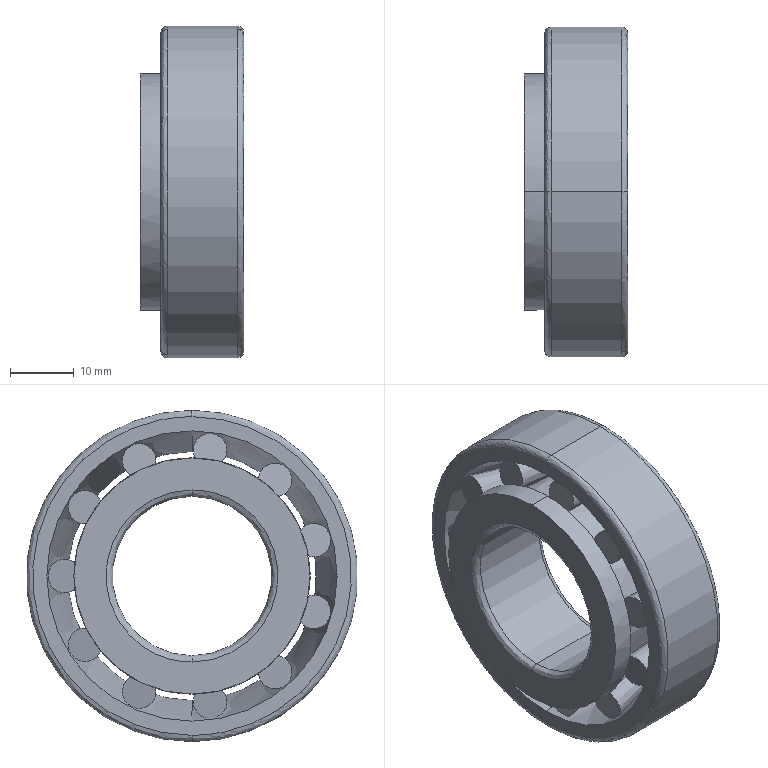Part | SolidWorks | features BaseBody 2 | 2 solids | 72 faces | box 16.25 x 52 x 52 mm | volume 17643 mm3 | cone 30 | plane 26 | spline 8 | cylinder 8 | commonest cylinder face diameters 25 x2 34.016 x2 37.07 x2 52 x2